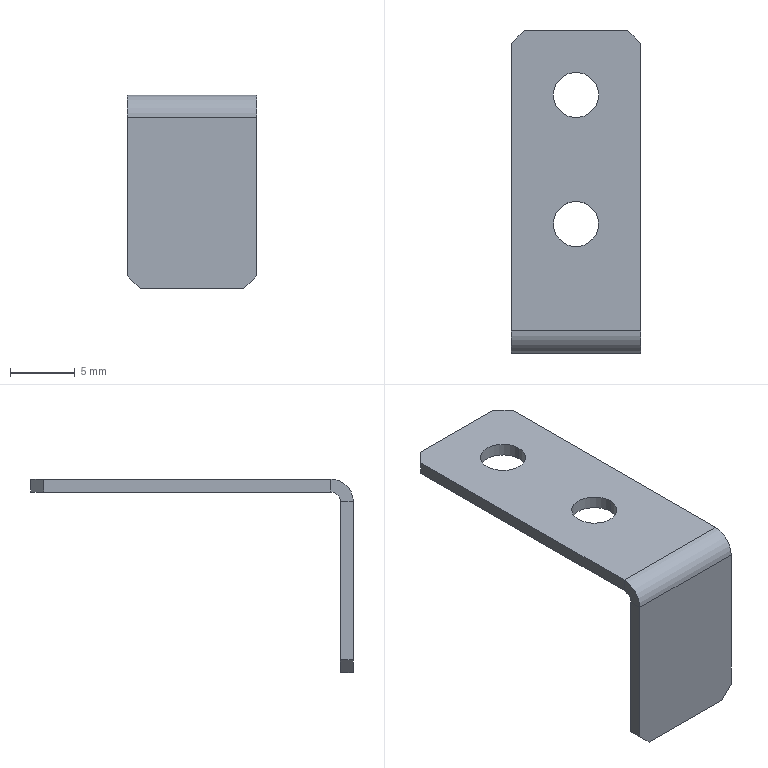Part | STEP file | PN_0006 BKT | 1 solid | 22 faces | box 10 x 25 x 15 mm | volume 363.45 mm3 | plane 16 | cylinder 6 | commonest cylinder face diameters 3.5 x4 1.473 x1 3.473 x1